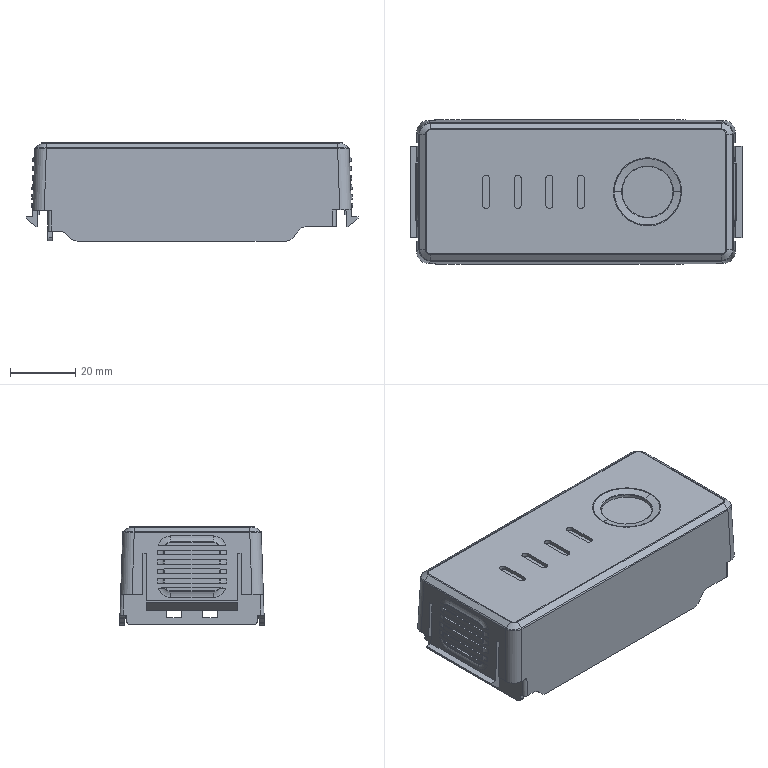Part | SolidWorks | features BaseBody 1 | 1 solid | 426 faces | box 101.5 x 44.3 x 30 mm | volume 74676 mm3 | plane 293 | cylinder 84 | spline 28 | cone 13 | torus 8 | commonest cylinder face diameters 1 x32 8 x20 2.2 x8 6 x8 2 x6 3.8 x4